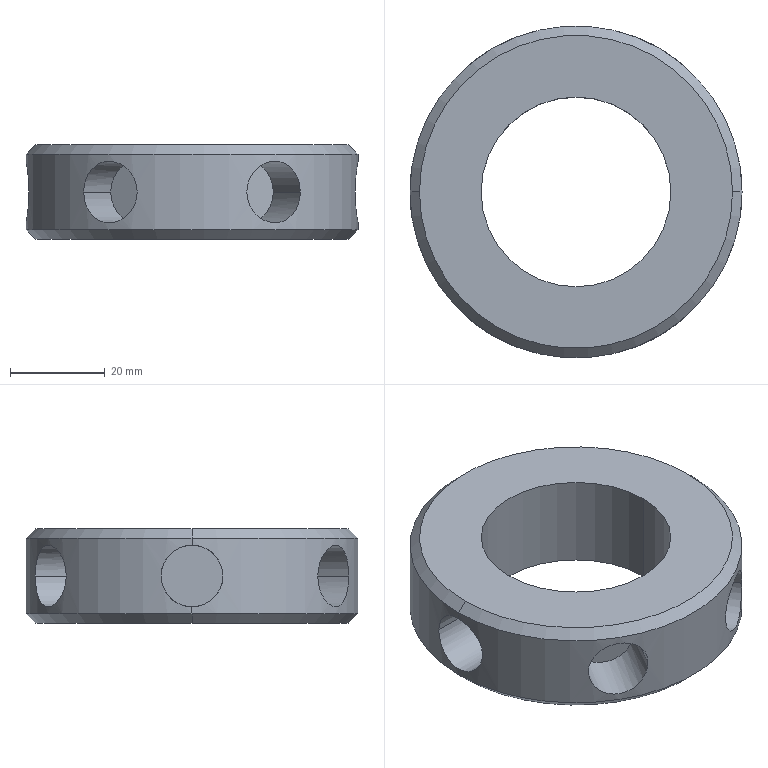Part | Creo | features CUT 6, DATUM PLANE 4, CURVE 2, CHAMFER 1, COORDINATE SYSTEM 1, PATTERN 1, PROTRUSION 1 | 1 solid | 28 faces | box 70 x 70 x 20 mm | volume 41537 mm3 | cylinder 16 | plane 8 | cone 4 | commonest cylinder face diameters 13 x12 40 x2 70 x2
STEP:
#1=CARTESIAN_POINT('',(0.,0.,0.));
#2=DIRECTION('',(0.,0.,1.));
#3=DIRECTION('',(1.,0.,0.));
#4=AXIS2_PLACEMENT_3D('',#1,#2,#3);
#5=CARTESIAN_POINT('',(-33.,0.,0.));
#6=VERTEX_POINT('',#5);
#7=CARTESIAN_POINT('',(33.,0.,0.));
#8=VERTEX_POINT('',#7);
#9=CARTESIAN_POINT('',(0.,0.,0.));
#10=DIRECTION('',(0.,0.,-1.));
#11=DIRECTION('',(-1.,0.,0.));
#12=AXIS2_PLACEMENT_3D('',#9,#10,#11);
#13=CIRCLE('',#12,33.);
#14=EDGE_CURVE('',#6,#8,#13,.T.);
#15=ORIENTED_EDGE('',*,*,#14,.F.);
#16=CARTESIAN_POINT('',(0.,0.,0.));
#17=DIRECTION('',(0.,0.,-1.));
#18=DIRECTION('',(1.,0.,0.));
#19=AXIS2_PLACEMENT_3D('',#16,#17,#18);
#20=CIRCLE('',#19,33.);
#21=EDGE_CURVE('',#8,#6,#20,.T.);
#22=ORIENTED_EDGE('',*,*,#21,.F.);
#23=EDGE_LOOP('',(#15,#22));
#24=FACE_OUTER_BOUND('',#23,.F.);
#25=CARTESIAN_POINT('',(20.,0.,0.));
#26=VERTEX_POINT('',#25);
#27=CARTESIAN_POINT('',(-20.,0.,0.));
#28=VERTEX_POINT('',#27);
#29=CARTESIAN_POINT('',(0.,0.,0.));
#30=DIRECTION('',(0.,0.,-1.));
#31=DIRECTION('',(1.,0.,0.));
#32=AXIS2_PLACEMENT_3D('',#29,#30,#31);
#33=CIRCLE('',#32,20.);
#34=EDGE_CURVE('',#26,#28,#33,.T.);
#35=ORIENTED_EDGE('',*,*,#34,.T.);
#36=CARTESIAN_POINT('',(0.,0.,0.));
#37=DIRECTION('',(0.,0.,-1.));
#38=DIRECTION('',(-1.,0.,0.));
#39=AXIS2_PLACEMENT_3D('',#36,#37,#38);
#40=CIRCLE('',#39,20.);
#41=EDGE_CURVE('',#28,#26,#40,.T.);
#42=ORIENTED_EDGE('',*,*,#41,.T.);
#43=EDGE_LOOP('',(#35,#42));
#44=FACE_BOUND('',#43,.F.);
#45=CARTESIAN_POINT('',(0.,0.,0.));
#46=DIRECTION('',(0.,0.,1.));
#47=DIRECTION('',(1.,0.,0.));
#48=AXIS2_PLACEMENT_3D('',#45,#46,#47);
#49=PLANE('',#48);
#50=ADVANCED_FACE('',(#24,#44),#49,.F.);
#51=ORIENTED_EDGE('',*,*,#34,.F.);
#52=CARTESIAN_POINT('',(20.,0.,20.));
#53=VERTEX_POINT('',#52);
#54=CARTESIAN_POINT('',(20.,0.,0.));
#55=DIRECTION('',(0.,0.,1.));
#56=VECTOR('',#55,20.);
#57=LINE('',#54,#56);
#58=EDGE_CURVE('',#26,#53,#57,.T.);
#59=ORIENTED_EDGE('',*,*,#58,.T.);
#60=CARTESIAN_POINT('',(-20.,0.,20.));
#61=VERTEX_POINT('',#60);
#62=CARTESIAN_POINT('',(0.,0.,20.));
#63=DIRECTION('',(0.,0.,-1.));
#64=DIRECTION('',(1.,0.,0.));
#65=AXIS2_PLACEMENT_3D('',#62,#63,#64);
#66=CIRCLE('',#65,20.);
#67=EDGE_CURVE('',#53,#61,#66,.T.);
#68=ORIENTED_EDGE('',*,*,#67,.T.);
#69=CARTESIAN_POINT('',(-20.,0.,0.));
#70=DIRECTION('',(0.,0.,1.));
#71=VECTOR('',#70,20.);
#72=LINE('',#69,#71);
#73=EDGE_CURVE('',#28,#61,#72,.T.);
#74=ORIENTED_EDGE('',*,*,#73,.F.);
#75=EDGE_LOOP('',(#51,#59,#68,#74));
#76=FACE_OUTER_BOUND('',#75,.F.);
#77=CARTESIAN_POINT('',(0.,0.,0.));
#78=DIRECTION('',(0.,0.,1.));
#79=DIRECTION('',(1.,0.,0.));
#80=AXIS2_PLACEMENT_3D('',#77,#78,#79);
#81=CYLINDRICAL_SURFACE('',#80,20.);
#82=ADVANCED_FACE('',(#76),#81,.F.);
#83=ORIENTED_EDGE('',*,*,#41,.F.);
#84=ORIENTED_EDGE('',*,*,#73,.T.);
#85=CARTESIAN_POINT('',(0.,0.,20.));
#86=DIRECTION('',(0.,0.,-1.));
#87=DIRECTION('',(-1.,0.,0.));
#88=AXIS2_PLACEMENT_3D('',#85,#86,#87);
#89=CIRCLE('',#88,20.);
#90=EDGE_CURVE('',#61,#53,#89,.T.);
#91=ORIENTED_EDGE('',*,*,#90,.T.);
#92=ORIENTED_EDGE('',*,*,#58,.F.);
#93=EDGE_LOOP('',(#83,#84,#91,#92));
#94=FACE_OUTER_BOUND('',#93,.F.);
#95=CARTESIAN_POINT('',(0.,0.,0.));
#96=DIRECTION('',(0.,0.,1.));
#97=DIRECTION('',(1.,0.,0.));
#98=AXIS2_PLACEMENT_3D('',#95,#96,#97);
#99=CYLINDRICAL_SURFACE('',#98,20.);
#100=ADVANCED_FACE('',(#94),#99,.F.);
#101=CARTESIAN_POINT('',(33.,0.,20.));
#102=VERTEX_POINT('',#101);
#103=CARTESIAN_POINT('',(-33.,0.,20.));
#104=VERTEX_POINT('',#103);
#105=CARTESIAN_POINT('',(0.,0.,20.));
#106=DIRECTION('',(0.,0.,1.));
#107=DIRECTION('',(1.,0.,0.));
#108=AXIS2_PLACEMENT_3D('',#105,#106,#107);
#109=CIRCLE('',#108,33.);
#110=EDGE_CURVE('',#102,#104,#109,.T.);
#111=ORIENTED_EDGE('',*,*,#110,.F.);
#112=CARTESIAN_POINT('',(0.,0.,20.));
#113=DIRECTION('',(0.,0.,1.));
#114=DIRECTION('',(-1.,0.,0.));
#115=AXIS2_PLACEMENT_3D('',#112,#113,#114);
#116=CIRCLE('',#115,33.);
#117=EDGE_CURVE('',#104,#102,#116,.T.);
#118=ORIENTED_EDGE('',*,*,#117,.F.);
#119=EDGE_LOOP('',(#111,#118));
#120=FACE_OUTER_BOUND('',#119,.F.);
#121=ORIENTED_EDGE('',*,*,#67,.F.);
#122=ORIENTED_EDGE('',*,*,#90,.F.);
#123=EDGE_LOOP('',(#121,#122));
#124=FACE_BOUND('',#123,.F.);
#125=CARTESIAN_POINT('',(0.,0.,20.));
#126=DIRECTION('',(0.,0.,1.));
#127=DIRECTION('',(1.,0.,0.));
#128=AXIS2_PLACEMENT_3D('',#125,#126,#127);
#129=PLANE('',#128);
#130=ADVANCED_FACE('',(#120,#124),#129,.T.);
#131=ORIENTED_EDGE('',*,*,#110,.T.);
#132=CARTESIAN_POINT('',(-35.,0.,18.));
#133=VERTEX_POINT('',#132);
#134=CARTESIAN_POINT('',(-33.,-0.000000004,20.));
#135=DIRECTION('',(-0.7071,0.,-0.7071));
#136=VECTOR('',#135,2.828);
#137=LINE('',#134,#136);
#138=EDGE_CURVE('',#104,#133,#137,.T.);
#139=ORIENTED_EDGE('',*,*,#138,.T.);
#140=CARTESIAN_POINT('',(35.,0.,18.));
#141=VERTEX_POINT('',#140);
#142=CARTESIAN_POINT('',(0.,0.,18.));
#143=DIRECTION('',(0.,0.,1.));
#144=DIRECTION('',(1.,0.,0.));
#145=AXIS2_PLACEMENT_3D('',#142,#143,#144);
#146=CIRCLE('',#145,35.);
#147=EDGE_CURVE('',#141,#133,#146,.T.);
#148=ORIENTED_EDGE('',*,*,#147,.F.);
#149=CARTESIAN_POINT('',(33.,0.000000004,20.));
#150=DIRECTION('',(0.7071,0.,-0.7071));
#151=VECTOR('',#150,2.828);
#152=LINE('',#149,#151);
#153=EDGE_CURVE('',#102,#141,#152,.T.);
#154=ORIENTED_EDGE('',*,*,#153,.F.);
#155=EDGE_LOOP('',(#131,#139,#148,#154));
#156=FACE_OUTER_BOUND('',#155,.F.);
#157=CARTESIAN_POINT('',(0.,0.,19.));
#158=DIRECTION('',(0.,0.,-1.));
#159=DIRECTION('',(0.,-1.,0.));
#160=AXIS2_PLACEMENT_3D('',#157,#158,#159);
#161=CONICAL_SURFACE('',#160,34.,45.);
#162=ADVANCED_FACE('',(#156),#161,.T.);
#163=ORIENTED_EDGE('',*,*,#117,.T.);
#164=ORIENTED_EDGE('',*,*,#153,.T.);
#165=CARTESIAN_POINT('',(0.,0.,18.));
#166=DIRECTION('',(0.,0.,1.));
#167=DIRECTION('',(-1.,0.,0.));
#168=AXIS2_PLACEMENT_3D('',#165,#166,#167);
#169=CIRCLE('',#168,35.);
#170=EDGE_CURVE('',#133,#141,#169,.T.);
#171=ORIENTED_EDGE('',*,*,#170,.F.);
#172=ORIENTED_EDGE('',*,*,#138,.F.);
#173=EDGE_LOOP('',(#163,#164,#171,#172));
#174=FACE_OUTER_BOUND('',#173,.F.);
#175=CARTESIAN_POINT('',(0.,0.,19.));
#176=DIRECTION('',(0.,0.,-1.));
#177=DIRECTION('',(0.,-1.,0.));
#178=AXIS2_PLACEMENT_3D('',#175,#176,#177);
#179=CONICAL_SURFACE('',#178,34.,45.);
#180=ADVANCED_FACE('',(#174),#179,.T.);
#181=CARTESIAN_POINT('',(35.,0.,2.));
#182=VERTEX_POINT('',#181);
#183=CARTESIAN_POINT('',(-35.,0.,2.));
#184=VERTEX_POINT('',#183);
#185=CARTESIAN_POINT('',(0.,0.,2.));
#186=DIRECTION('',(0.,0.,-1.));
#187=DIRECTION('',(1.,0.,0.));
#188=AXIS2_PLACEMENT_3D('',#185,#186,#187);
#189=CIRCLE('',#188,35.);
#190=EDGE_CURVE('',#182,#184,#189,.T.);
#191=ORIENTED_EDGE('',*,*,#190,.T.);
#192=CARTESIAN_POINT('',(-35.,0.,3.5));
#193=VERTEX_POINT('',#192);
#194=CARTESIAN_POINT('',(-35.,-0.000000003,2.));
#195=DIRECTION('',(0.,0.000000002,1.));
#196=VECTOR('',#195,1.5);
#197=LINE('',#194,#196);
#198=EDGE_CURVE('',#184,#193,#197,.T.);
#199=ORIENTED_EDGE('',*,*,#198,.T.);
#200=CARTESIAN_POINT('',(-34.391,-6.5,10.));
#201=VERTEX_POINT('',#200);
#202=CARTESIAN_POINT('',(-34.391,-6.5,9.619));
#203=CARTESIAN_POINT('',(-34.404,-6.434,8.869));
#204=CARTESIAN_POINT('',(-34.458,-6.137,7.76));
#205=CARTESIAN_POINT('',(-34.541,-5.658,6.734));
#206=CARTESIAN_POINT('',(-34.643,-5.001,5.796));
#207=CARTESIAN_POINT('',(-34.75,-4.205,5.001));
#208=CARTESIAN_POINT('',(-34.852,-3.269,4.343));
#209=CARTESIAN_POINT('',(-34.934,-2.239,3.862));
#210=CARTESIAN_POINT('',(-34.988,-1.113,3.562));
#211=CARTESIAN_POINT('',(-35.,-0.3734,3.5));
#212=CARTESIAN_POINT('',(-35.,0.,3.5));
#213=B_SPLINE_CURVE_WITH_KNOTS('',3,(#200,#202,#203,#204,#205,#206,#207,#208,#209,#210,#211,#212),.UNSPECIFIED.,.F.,.F.,(4,1,1,1,1,1,1,1,1,4),(0.,0.1111,0.2222,0.3333,0.4444,0.5556,0.6667,0.7778,0.8889,1.),.UNSPECIFIED.);
#214=EDGE_CURVE('',#201,#193,#213,.T.);
#215=ORIENTED_EDGE('',*,*,#214,.F.);
#216=CARTESIAN_POINT('',(-35.,0.,16.5));
#217=VERTEX_POINT('',#216);
#218=CARTESIAN_POINT('',(-35.,0.,16.5));
#219=CARTESIAN_POINT('',(-35.,-0.422,16.5));
#220=CARTESIAN_POINT('',(-34.985,-1.254,16.421));
#221=CARTESIAN_POINT('',(-34.917,-2.511,16.042));
#222=CARTESIAN_POINT('',(-34.816,-3.639,15.436));
#223=CARTESIAN_POINT('',(-34.697,-4.626,14.625));
#224=CARTESIAN_POINT('',(-34.578,-5.437,13.638));
#225=CARTESIAN_POINT('',(-34.476,-6.043,12.507));
#226=CARTESIAN_POINT('',(-34.407,-6.416,11.273));
#227=CARTESIAN_POINT('',(-34.391,-6.5,10.43));
#228=CARTESIAN_POINT('',(-34.391,-6.5,10.));
#229=B_SPLINE_CURVE_WITH_KNOTS('',3,(#218,#219,#220,#221,#222,#223,#224,#225,#226,#227,#228),.UNSPECIFIED.,.F.,.F.,(4,1,1,1,1,1,1,1,4),(0.,0.125,0.25,0.375,0.5,0.625,0.75,0.875,1.),.UNSPECIFIED.);
#230=EDGE_CURVE('',#217,#201,#229,.T.);
#231=ORIENTED_EDGE('',*,*,#230,.F.);
#232=CARTESIAN_POINT('',(-35.,0.,16.5));
#233=DIRECTION('',(0.,-0.000000002,1.));
#234=VECTOR('',#233,1.5);
#235=LINE('',#232,#234);
#236=EDGE_CURVE('',#217,#133,#235,.T.);
#237=ORIENTED_EDGE('',*,*,#236,.T.);
#238=ORIENTED_EDGE('',*,*,#170,.T.);
#239=CARTESIAN_POINT('',(35.,0.,16.5));
#240=VERTEX_POINT('',#239);
#241=CARTESIAN_POINT('',(35.,0.,16.5));
#242=DIRECTION('',(0.,0.000000002,1.));
#243=VECTOR('',#242,1.5);
#244=LINE('',#241,#243);
#245=EDGE_CURVE('',#240,#141,#244,.T.);
#246=ORIENTED_EDGE('',*,*,#245,.F.);
#247=CARTESIAN_POINT('',(34.391,-6.5,10.));
#248=VERTEX_POINT('',#247);
#249=CARTESIAN_POINT('',(34.391,-6.5,10.));
#250=CARTESIAN_POINT('',(34.391,-6.5,10.381));
#251=CARTESIAN_POINT('',(34.404,-6.434,11.131));
#252=CARTESIAN_POINT('',(34.458,-6.137,12.24));
#253=CARTESIAN_POINT('',(34.541,-5.658,13.266));
#254=CARTESIAN_POINT('',(34.643,-5.001,14.204));
#255=CARTESIAN_POINT('',(34.75,-4.205,14.999));
#256=CARTESIAN_POINT('',(34.852,-3.269,15.657));
#257=CARTESIAN_POINT('',(34.934,-2.239,16.138));
#258=CARTESIAN_POINT('',(34.988,-1.113,16.438));
#259=CARTESIAN_POINT('',(35.,-0.3732,16.5));
#260=CARTESIAN_POINT('',(35.,0.,16.5));
#261=B_SPLINE_CURVE_WITH_KNOTS('',3,(#249,#250,#251,#252,#253,#254,#255,#256,#257,#258,#259,#260),.UNSPECIFIED.,.F.,.F.,(4,1,1,1,1,1,1,1,1,4),(0.,0.1111,0.2222,0.3333,0.4444,0.5556,0.6667,0.7778,0.8889,1.),.UNSPECIFIED.);
#262=EDGE_CURVE('',#248,#240,#261,.T.);
#263=ORIENTED_EDGE('',*,*,#262,.F.);
#264=CARTESIAN_POINT('',(35.,0.,3.5));
#265=VERTEX_POINT('',#264);
#266=CARTESIAN_POINT('',(35.,0.,3.5));
#267=CARTESIAN_POINT('',(35.,-0.4219,3.5));
#268=CARTESIAN_POINT('',(34.985,-1.254,3.579));
#269=CARTESIAN_POINT('',(34.917,-2.511,3.958));
#270=CARTESIAN_POINT('',(34.816,-3.639,4.564));
#271=CARTESIAN_POINT('',(34.697,-4.626,5.375));
#272=CARTESIAN_POINT('',(34.578,-5.437,6.363));
#273=CARTESIAN_POINT('',(34.476,-6.043,7.493));
#274=CARTESIAN_POINT('',(34.407,-6.416,8.727));
#275=CARTESIAN_POINT('',(34.391,-6.5,9.57));
#276=B_SPLINE_CURVE_WITH_KNOTS('',3,(#266,#267,#268,#269,#270,#271,#272,#273,#274,#275,#247),.UNSPECIFIED.,.F.,.F.,(4,1,1,1,1,1,1,1,4),(0.,0.125,0.25,0.375,0.5,0.625,0.75,0.875,1.),.UNSPECIFIED.);
#277=EDGE_CURVE('',#265,#248,#276,.T.);
#278=ORIENTED_EDGE('',*,*,#277,.F.);
#279=CARTESIAN_POINT('',(35.,0.000000003,2.));
#280=DIRECTION('',(0.,-0.000000002,1.));
#281=VECTOR('',#280,1.5);
#282=LINE('',#279,#281);
#283=EDGE_CURVE('',#182,#265,#282,.T.);
#284=ORIENTED_EDGE('',*,*,#283,.F.);
#285=EDGE_LOOP('',(#191,#199,#215,#231,#237,#238,#246,#263,#278,#284));
#286=FACE_OUTER_BOUND('',#285,.F.);
#287=CARTESIAN_POINT('',(11.566,-33.034,10.));
#288=VERTEX_POINT('',#287);
#289=CARTESIAN_POINT('',(22.825,-26.534,10.));
#290=VERTEX_POINT('',#289);
#291=CARTESIAN_POINT('',(11.566,-33.034,9.544));
#292=CARTESIAN_POINT('',(11.657,-33.002,8.651));
#293=CARTESIAN_POINT('',(12.058,-32.859,7.348));
#294=CARTESIAN_POINT('',(12.708,-32.615,6.158));
#295=CARTESIAN_POINT('',(13.572,-32.267,5.132));
#296=CARTESIAN_POINT('',(14.6,-31.817,4.324));
#297=CARTESIAN_POINT('',(15.733,-31.274,3.769));
#298=CARTESIAN_POINT('',(16.913,-30.652,3.488));
#299=CARTESIAN_POINT('',(18.089,-29.973,3.488));
#300=CARTESIAN_POINT('',(19.218,-29.262,3.769));
#301=CARTESIAN_POINT('',(20.254,-28.552,4.324));
#302=CARTESIAN_POINT('',(21.158,-27.887,5.132));
#303=CARTESIAN_POINT('',(21.892,-27.313,6.158));
#304=CARTESIAN_POINT('',(22.428,-26.872,7.348));
#305=CARTESIAN_POINT('',(22.752,-26.596,8.651));
#306=CARTESIAN_POINT('',(22.825,-26.534,9.544));
#307=B_SPLINE_CURVE_WITH_KNOTS('',3,(#287,#291,#292,#293,#294,#295,#296,#297,#298,#299,#300,#301,#302,#303,#304,#305,#306,#289),.UNSPECIFIED.,.F.,.F.,(4,1,1,1,1,1,1,1,1,1,1,1,1,1,1,4),(0.,0.06667,0.1333,0.2,0.2667,0.3333,0.4,0.4667,0.5333,0.6,0.6667,0.7333,0.8,0.8667,0.9333,1.),.UNSPECIFIED.);
#308=EDGE_CURVE('',#288,#290,#307,.T.);
#309=ORIENTED_EDGE('',*,*,#308,.T.);
#310=CARTESIAN_POINT('',(22.825,-26.534,10.));
#311=CARTESIAN_POINT('',(22.825,-26.534,10.456));
#312=CARTESIAN_POINT('',(22.752,-26.596,11.349));
#313=CARTESIAN_POINT('',(22.428,-26.872,12.652));
#314=CARTESIAN_POINT('',(21.892,-27.313,13.842));
#315=CARTESIAN_POINT('',(21.158,-27.887,14.868));
#316=CARTESIAN_POINT('',(20.254,-28.552,15.676));
#317=CARTESIAN_POINT('',(19.218,-29.262,16.231));
#318=CARTESIAN_POINT('',(18.089,-29.973,16.512));
#319=CARTESIAN_POINT('',(16.913,-30.652,16.512));
#320=CARTESIAN_POINT('',(15.733,-31.274,16.231));
#321=CARTESIAN_POINT('',(14.6,-31.817,15.676));
#322=CARTESIAN_POINT('',(13.572,-32.267,14.868));
#323=CARTESIAN_POINT('',(12.708,-32.615,13.842));
#324=CARTESIAN_POINT('',(12.058,-32.859,12.652));
#325=CARTESIAN_POINT('',(11.657,-33.002,11.349));
#326=CARTESIAN_POINT('',(11.566,-33.034,10.456));
#327=CARTESIAN_POINT('',(11.566,-33.034,10.));
#328=B_SPLINE_CURVE_WITH_KNOTS('',3,(#310,#311,#312,#313,#314,#315,#316,#317,#318,#319,#320,#321,#322,#323,#324,#325,#326,#327),.UNSPECIFIED.,.F.,.F.,(4,1,1,1,1,1,1,1,1,1,1,1,1,1,1,4),(0.,0.06667,0.1333,0.2,0.2667,0.3333,0.4,0.4667,0.5333,0.6,0.6667,0.7333,0.8,0.8667,0.9333,1.),.UNSPECIFIED.);
#329=EDGE_CURVE('',#290,#288,#328,.T.);
#330=ORIENTED_EDGE('',*,*,#329,.T.);
#331=EDGE_LOOP('',(#309,#330));
#332=FACE_BOUND('',#331,.F.);
#333=CARTESIAN_POINT('',(-22.825,-26.534,10.));
#334=VERTEX_POINT('',#333);
#335=CARTESIAN_POINT('',(-11.566,-33.034,10.));
#336=VERTEX_POINT('',#335);
#337=CARTESIAN_POINT('',(-22.825,-26.534,9.544));
#338=CARTESIAN_POINT('',(-22.752,-26.596,8.651));
#339=CARTESIAN_POINT('',(-22.428,-26.872,7.348));
#340=CARTESIAN_POINT('',(-21.892,-27.313,6.158));
#341=CARTESIAN_POINT('',(-21.158,-27.887,5.132));
#342=CARTESIAN_POINT('',(-20.254,-28.552,4.324));
#343=CARTESIAN_POINT('',(-19.218,-29.262,3.769));
#344=CARTESIAN_POINT('',(-18.089,-29.973,3.488));
#345=CARTESIAN_POINT('',(-16.913,-30.652,3.488));
#346=CARTESIAN_POINT('',(-15.733,-31.274,3.769));
#347=CARTESIAN_POINT('',(-14.6,-31.817,4.324));
#348=CARTESIAN_POINT('',(-13.572,-32.267,5.132));
#349=CARTESIAN_POINT('',(-12.708,-32.615,6.158));
#350=CARTESIAN_POINT('',(-12.058,-32.859,7.348));
#351=CARTESIAN_POINT('',(-11.657,-33.002,8.651));
#352=CARTESIAN_POINT('',(-11.566,-33.034,9.544));
#353=B_SPLINE_CURVE_WITH_KNOTS('',3,(#333,#337,#338,#339,#340,#341,#342,#343,#344,#345,#346,#347,#348,#349,#350,#351,#352,#335),.UNSPECIFIED.,.F.,.F.,(4,1,1,1,1,1,1,1,1,1,1,1,1,1,1,4),(0.,0.06667,0.1333,0.2,0.2667,0.3333,0.4,0.4667,0.5333,0.6,0.6667,0.7333,0.8,0.8667,0.9333,1.),.UNSPECIFIED.);
#354=EDGE_CURVE('',#334,#336,#353,.T.);
#355=ORIENTED_EDGE('',*,*,#354,.T.);
#356=CARTESIAN_POINT('',(-11.566,-33.034,10.));
#357=CARTESIAN_POINT('',(-11.566,-33.034,10.456));
#358=CARTESIAN_POINT('',(-11.657,-33.002,11.349));
#359=CARTESIAN_POINT('',(-12.058,-32.859,12.652));
#360=CARTESIAN_POINT('',(-12.708,-32.615,13.842));
#361=CARTESIAN_POINT('',(-13.572,-32.267,14.868));
#362=CARTESIAN_POINT('',(-14.6,-31.817,15.676));
#363=CARTESIAN_POINT('',(-15.733,-31.274,16.231));
#364=CARTESIAN_POINT('',(-16.913,-30.652,16.512));
#365=CARTESIAN_POINT('',(-18.089,-29.973,16.512));
#366=CARTESIAN_POINT('',(-19.218,-29.262,16.231));
#367=CARTESIAN_POINT('',(-20.254,-28.552,15.676));
#368=CARTESIAN_POINT('',(-21.158,-27.887,14.868));
#369=CARTESIAN_POINT('',(-21.892,-27.313,13.842));
#370=CARTESIAN_POINT('',(-22.428,-26.872,12.652));
#371=CARTESIAN_POINT('',(-22.752,-26.596,11.349));
#372=CARTESIAN_POINT('',(-22.825,-26.534,10.456));
#373=CARTESIAN_POINT('',(-22.825,-26.534,10.));
#374=B_SPLINE_CURVE_WITH_KNOTS('',3,(#356,#357,#358,#359,#360,#361,#362,#363,#364,#365,#366,#367,#368,#369,#370,#371,#372,#373),.UNSPECIFIED.,.F.,.F.,(4,1,1,1,1,1,1,1,1,1,1,1,1,1,1,4),(0.,0.06667,0.1333,0.2,0.2667,0.3333,0.4,0.4667,0.5333,0.6,0.6667,0.7333,0.8,0.8667,0.9333,1.),.UNSPECIFIED.);
#375=EDGE_CURVE('',#336,#334,#374,.T.);
#376=ORIENTED_EDGE('',*,*,#375,.T.);
#377=EDGE_LOOP('',(#355,#376));
#378=FACE_BOUND('',#377,.F.);
#379=CARTESIAN_POINT('',(0.,0.,0.));
#380=DIRECTION('',(0.,0.,1.));
#381=DIRECTION('',(1.,0.,0.));
#382=AXIS2_PLACEMENT_3D('',#379,#380,#381);
#383=CYLINDRICAL_SURFACE('',#382,35.);
#384=ADVANCED_FACE('',(#286,#332,#378),#383,.T.);
#385=ORIENTED_EDGE('',*,*,#354,.F.);
#386=CARTESIAN_POINT('',(-17.129,-16.669,10.));
#387=VERTEX_POINT('',#386);
#388=CARTESIAN_POINT('',(-22.825,-26.534,10.));
#389=DIRECTION('',(0.5,0.866,0.));
#390=VECTOR('',#389,11.391);
#391=LINE('',#388,#390);
#392=EDGE_CURVE('',#334,#387,#391,.T.);
#393=ORIENTED_EDGE('',*,*,#392,.T.);
#394=CARTESIAN_POINT('',(-5.871,-23.169,10.));
#395=VERTEX_POINT('',#394);
#396=CARTESIAN_POINT('',(-11.5,-19.919,10.));
#397=DIRECTION('',(-0.5,-0.866,0.));
#398=DIRECTION('',(-0.866,0.5,0.));
#399=AXIS2_PLACEMENT_3D('',#396,#397,#398);
#400=CIRCLE('',#399,6.5);
#401=EDGE_CURVE('',#387,#395,#400,.T.);
#402=ORIENTED_EDGE('',*,*,#401,.T.);
#403=CARTESIAN_POINT('',(-11.566,-33.034,10.));
#404=DIRECTION('',(0.5,0.866,0.));
#405=VECTOR('',#404,11.391);
#406=LINE('',#403,#405);
#407=EDGE_CURVE('',#336,#395,#406,.T.);
#408=ORIENTED_EDGE('',*,*,#407,.F.);
#409=EDGE_LOOP('',(#385,#393,#402,#408));
#410=FACE_OUTER_BOUND('',#409,.F.);
#411=CARTESIAN_POINT('',(-17.5,-30.311,10.));
#412=DIRECTION('',(-0.5,-0.866,0.));
#413=DIRECTION('',(-0.866,0.5,0.));
#414=AXIS2_PLACEMENT_3D('',#411,#412,#413);
#415=CYLINDRICAL_SURFACE('',#414,6.5);
#416=ADVANCED_FACE('',(#410),#415,.F.);
#417=ORIENTED_EDGE('',*,*,#375,.F.);
#418=ORIENTED_EDGE('',*,*,#407,.T.);
#419=CARTESIAN_POINT('',(-11.5,-19.919,10.));
#420=DIRECTION('',(-0.5,-0.866,0.));
#421=DIRECTION('',(0.866,-0.5,0.));
#422=AXIS2_PLACEMENT_3D('',#419,#420,#421);
#423=CIRCLE('',#422,6.5);
#424=EDGE_CURVE('',#395,#387,#423,.T.);
#425=ORIENTED_EDGE('',*,*,#424,.T.);
#426=ORIENTED_EDGE('',*,*,#392,.F.);
#427=EDGE_LOOP('',(#417,#418,#425,#426));
#428=FACE_OUTER_BOUND('',#427,.F.);
#429=CARTESIAN_POINT('',(-17.5,-30.311,10.));
#430=DIRECTION('',(-0.5,-0.866,0.));
#431=DIRECTION('',(-0.866,0.5,0.));
#432=AXIS2_PLACEMENT_3D('',#429,#430,#431);
#433=CYLINDRICAL_SURFACE('',#432,6.5);
#434=ADVANCED_FACE('',(#428),#433,.F.);
#435=ORIENTED_EDGE('',*,*,#401,.F.);
#436=ORIENTED_EDGE('',*,*,#424,.F.);
#437=EDGE_LOOP('',(#435,#436));
#438=FACE_OUTER_BOUND('',#437,.F.);
#439=CARTESIAN_POINT('',(-11.5,-19.919,0.));
#440=DIRECTION('',(-0.5,-0.866,0.));
#441=DIRECTION('',(-0.866,0.5,0.));
#442=AXIS2_PLACEMENT_3D('',#439,#440,#441);
#443=PLANE('',#442);
#444=ADVANCED_FACE('',(#438),#443,.T.);
#445=ORIENTED_EDGE('',*,*,#308,.F.);
#446=CARTESIAN_POINT('',(5.871,-23.169,10.));
#447=VERTEX_POINT('',#446);
#448=CARTESIAN_POINT('',(11.566,-33.034,10.));
#449=DIRECTION('',(-0.5,0.866,0.));
#450=VECTOR('',#449,11.391);
#451=LINE('',#448,#450);
#452=EDGE_CURVE('',#288,#447,#451,.T.);
#453=ORIENTED_EDGE('',*,*,#452,.T.);
#454=CARTESIAN_POINT('',(17.129,-16.669,10.));
#455=VERTEX_POINT('',#454);
#456=CARTESIAN_POINT('',(11.5,-19.919,10.));
#457=DIRECTION('',(0.5,-0.866,0.));
#458=DIRECTION('',(-0.866,-0.5,0.));
#459=AXIS2_PLACEMENT_3D('',#456,#457,#458);
#460=CIRCLE('',#459,6.5);
#461=EDGE_CURVE('',#447,#455,#460,.T.);
#462=ORIENTED_EDGE('',*,*,#461,.T.);
#463=CARTESIAN_POINT('',(22.825,-26.534,10.));
#464=DIRECTION('',(-0.5,0.866,0.));
#465=VECTOR('',#464,11.391);
#466=LINE('',#463,#465);
#467=EDGE_CURVE('',#290,#455,#466,.T.);
#468=ORIENTED_EDGE('',*,*,#467,.F.);
#469=EDGE_LOOP('',(#445,#453,#462,#468));
#470=FACE_OUTER_BOUND('',#469,.F.);
#471=CARTESIAN_POINT('',(17.5,-30.311,10.));
#472=DIRECTION('',(0.5,-0.866,0.));
#473=DIRECTION('',(-0.866,-0.5,0.));
#474=AXIS2_PLACEMENT_3D('',#471,#472,#473);
#475=CYLINDRICAL_SURFACE('',#474,6.5);
#476=ADVANCED_FACE('',(#470),#475,.F.);
#477=ORIENTED_EDGE('',*,*,#329,.F.);
#478=ORIENTED_EDGE('',*,*,#467,.T.);
#479=CARTESIAN_POINT('',(11.5,-19.919,10.));
#480=DIRECTION('',(0.5,-0.866,0.));
#481=DIRECTION('',(0.866,0.5,0.));
#482=AXIS2_PLACEMENT_3D('',#479,#480,#481);
#483=CIRCLE('',#482,6.5);
#484=EDGE_CURVE('',#455,#447,#483,.T.);
#485=ORIENTED_EDGE('',*,*,#484,.T.);
#486=ORIENTED_EDGE('',*,*,#452,.F.);
#487=EDGE_LOOP('',(#477,#478,#485,#486));
#488=FACE_OUTER_BOUND('',#487,.F.);
#489=CARTESIAN_POINT('',(17.5,-30.311,10.));
#490=DIRECTION('',(0.5,-0.866,0.));
#491=DIRECTION('',(-0.866,-0.5,0.));
#492=AXIS2_PLACEMENT_3D('',#489,#490,#491);
#493=CYLINDRICAL_SURFACE('',#492,6.5);
#494=ADVANCED_FACE('',(#488),#493,.F.);
#495=ORIENTED_EDGE('',*,*,#461,.F.);
#496=ORIENTED_EDGE('',*,*,#484,.F.);
#497=EDGE_LOOP('',(#495,#496));
#498=FACE_OUTER_BOUND('',#497,.F.);
#499=CARTESIAN_POINT('',(11.5,-19.919,0.));
#500=DIRECTION('',(0.5,-0.866,0.));
#501=DIRECTION('',(-0.866,-0.5,0.));
#502=AXIS2_PLACEMENT_3D('',#499,#500,#501);
#503=PLANE('',#502);
#504=ADVANCED_FACE('',(#498),#503,.T.);
#505=ORIENTED_EDGE('',*,*,#21,.T.);
#506=CARTESIAN_POINT('',(-33.,-0.000000004,0.));
#507=DIRECTION('',(-0.7071,0.,0.7071));
#508=VECTOR('',#507,2.828);
#509=LINE('',#506,#508);
#510=EDGE_CURVE('',#6,#184,#509,.T.);
#511=ORIENTED_EDGE('',*,*,#510,.T.);
#512=ORIENTED_EDGE('',*,*,#190,.F.);
#513=CARTESIAN_POINT('',(33.,0.000000004,0.));
#514=DIRECTION('',(0.7071,0.,0.7071));
#515=VECTOR('',#514,2.828);
#516=LINE('',#513,#515);
#517=EDGE_CURVE('',#8,#182,#516,.T.);
#518=ORIENTED_EDGE('',*,*,#517,.F.);
#519=EDGE_LOOP('',(#505,#511,#512,#518));
#520=FACE_OUTER_BOUND('',#519,.F.);
#521=CARTESIAN_POINT('',(0.,0.,1.));
#522=DIRECTION('',(0.,0.,1.));
#523=DIRECTION('',(0.,-1.,0.));
#524=AXIS2_PLACEMENT_3D('',#521,#522,#523);
#525=CONICAL_SURFACE('',#524,34.,45.);
#526=ADVANCED_FACE('',(#520),#525,.T.);
#527=ORIENTED_EDGE('',*,*,#14,.T.);
#528=ORIENTED_EDGE('',*,*,#517,.T.);
#529=CARTESIAN_POINT('',(0.,0.,2.));
#530=DIRECTION('',(0.,0.,-1.));
#531=DIRECTION('',(-1.,0.,0.));
#532=AXIS2_PLACEMENT_3D('',#529,#530,#531);
#533=CIRCLE('',#532,35.);
#534=EDGE_CURVE('',#184,#182,#533,.T.);
#535=ORIENTED_EDGE('',*,*,#534,.F.);
#536=ORIENTED_EDGE('',*,*,#510,.F.);
#537=EDGE_LOOP('',(#527,#528,#535,#536));
#538=FACE_OUTER_BOUND('',#537,.F.);
#539=CARTESIAN_POINT('',(0.,0.,1.));
#540=DIRECTION('',(0.,0.,1.));
#541=DIRECTION('',(0.,-1.,0.));
#542=AXIS2_PLACEMENT_3D('',#539,#540,#541);
#543=CONICAL_SURFACE('',#542,34.,45.);
#544=ADVANCED_FACE('',(#538),#543,.T.);
#545=ORIENTED_EDGE('',*,*,#534,.T.);
#546=ORIENTED_EDGE('',*,*,#283,.T.);
#547=CARTESIAN_POINT('',(34.391,6.5,10.));
#548=VERTEX_POINT('',#547);
#549=CARTESIAN_POINT('',(34.391,6.5,9.619));
#550=CARTESIAN_POINT('',(34.404,6.434,8.869));
#551=CARTESIAN_POINT('',(34.458,6.137,7.76));
#552=CARTESIAN_POINT('',(34.541,5.658,6.734));
#553=CARTESIAN_POINT('',(34.643,5.001,5.796));
#554=CARTESIAN_POINT('',(34.75,4.205,5.001));
#555=CARTESIAN_POINT('',(34.852,3.269,4.343));
#556=CARTESIAN_POINT('',(34.934,2.239,3.862));
#557=CARTESIAN_POINT('',(34.988,1.113,3.562));
#558=CARTESIAN_POINT('',(35.,0.3734,3.5));
#559=B_SPLINE_CURVE_WITH_KNOTS('',3,(#547,#549,#550,#551,#552,#553,#554,#555,#556,#557,#558,#264),.UNSPECIFIED.,.F.,.F.,(4,1,1,1,1,1,1,1,1,4),(0.,0.1111,0.2222,0.3333,0.4444,0.5556,0.6667,0.7778,0.8889,1.),.UNSPECIFIED.);
#560=EDGE_CURVE('',#548,#265,#559,.T.);
#561=ORIENTED_EDGE('',*,*,#560,.F.);
#562=CARTESIAN_POINT('',(35.,0.422,16.5));
#563=CARTESIAN_POINT('',(34.985,1.254,16.421));
#564=CARTESIAN_POINT('',(34.917,2.511,16.042));
#565=CARTESIAN_POINT('',(34.816,3.639,15.436));
#566=CARTESIAN_POINT('',(34.697,4.626,14.625));
#567=CARTESIAN_POINT('',(34.578,5.437,13.638));
#568=CARTESIAN_POINT('',(34.476,6.043,12.507));
#569=CARTESIAN_POINT('',(34.407,6.416,11.273));
#570=CARTESIAN_POINT('',(34.391,6.5,10.43));
#571=CARTESIAN_POINT('',(34.391,6.5,10.));
#572=B_SPLINE_CURVE_WITH_KNOTS('',3,(#239,#562,#563,#564,#565,#566,#567,#568,#569,#570,#571),.UNSPECIFIED.,.F.,.F.,(4,1,1,1,1,1,1,1,4),(0.,0.125,0.25,0.375,0.5,0.625,0.75,0.875,1.),.UNSPECIFIED.);
#573=EDGE_CURVE('',#240,#548,#572,.T.);
#574=ORIENTED_EDGE('',*,*,#573,.F.);
#575=ORIENTED_EDGE('',*,*,#245,.T.);
#576=ORIENTED_EDGE('',*,*,#147,.T.);
#577=ORIENTED_EDGE('',*,*,#236,.F.);
#578=CARTESIAN_POINT('',(-34.391,6.5,10.));
#579=VERTEX_POINT('',#578);
#580=CARTESIAN_POINT('',(-34.391,6.5,10.));
#581=CARTESIAN_POINT('',(-34.391,6.5,10.381));
#582=CARTESIAN_POINT('',(-34.404,6.434,11.131));
#583=CARTESIAN_POINT('',(-34.458,6.137,12.24));
#584=CARTESIAN_POINT('',(-34.541,5.658,13.266));
#585=CARTESIAN_POINT('',(-34.643,5.001,14.204));
#586=CARTESIAN_POINT('',(-34.75,4.205,14.999));
#587=CARTESIAN_POINT('',(-34.852,3.269,15.657));
#588=CARTESIAN_POINT('',(-34.934,2.239,16.138));
#589=CARTESIAN_POINT('',(-34.988,1.113,16.438));
#590=CARTESIAN_POINT('',(-35.,0.3732,16.5));
#591=B_SPLINE_CURVE_WITH_KNOTS('',3,(#580,#581,#582,#583,#584,#585,#586,#587,#588,#589,#590,#216),.UNSPECIFIED.,.F.,.F.,(4,1,1,1,1,1,1,1,1,4),(0.,0.1111,0.2222,0.3333,0.4444,0.5556,0.6667,0.7778,0.8889,1.),.UNSPECIFIED.);
#592=EDGE_CURVE('',#579,#217,#591,.T.);
#593=ORIENTED_EDGE('',*,*,#592,.F.);
#594=CARTESIAN_POINT('',(-35.,0.4219,3.5));
#595=CARTESIAN_POINT('',(-34.985,1.254,3.579));
#596=CARTESIAN_POINT('',(-34.917,2.511,3.958));
#597=CARTESIAN_POINT('',(-34.816,3.639,4.564));
#598=CARTESIAN_POINT('',(-34.697,4.626,5.375));
#599=CARTESIAN_POINT('',(-34.578,5.437,6.363));
#600=CARTESIAN_POINT('',(-34.476,6.043,7.493));
#601=CARTESIAN_POINT('',(-34.407,6.416,8.727));
#602=CARTESIAN_POINT('',(-34.391,6.5,9.57));
#603=B_SPLINE_CURVE_WITH_KNOTS('',3,(#192,#594,#595,#596,#597,#598,#599,#600,#601,#602,#578),.UNSPECIFIED.,.F.,.F.,(4,1,1,1,1,1,1,1,4),(0.,0.125,0.25,0.375,0.5,0.625,0.75,0.875,1.),.UNSPECIFIED.);
#604=EDGE_CURVE('',#193,#579,#603,.T.);
#605=ORIENTED_EDGE('',*,*,#604,.F.);
#606=ORIENTED_EDGE('',*,*,#198,.F.);
#607=EDGE_LOOP('',(#545,#546,#561,#574,#575,#576,#577,#593,#605,#606));
#608=FACE_OUTER_BOUND('',#607,.F.);
#609=CARTESIAN_POINT('',(-11.566,33.034,10.));
#610=VERTEX_POINT('',#609);
#611=CARTESIAN_POINT('',(-22.825,26.534,10.));
#612=VERTEX_POINT('',#611);
#613=CARTESIAN_POINT('',(-11.566,33.034,9.544));
#614=CARTESIAN_POINT('',(-11.657,33.002,8.651));
#615=CARTESIAN_POINT('',(-12.058,32.859,7.348));
#616=CARTESIAN_POINT('',(-12.708,32.615,6.158));
#617=CARTESIAN_POINT('',(-13.572,32.267,5.132));
#618=CARTESIAN_POINT('',(-14.6,31.817,4.324));
#619=CARTESIAN_POINT('',(-15.733,31.274,3.769));
#620=CARTESIAN_POINT('',(-16.913,30.652,3.488));
#621=CARTESIAN_POINT('',(-18.089,29.973,3.488));
#622=CARTESIAN_POINT('',(-19.218,29.262,3.769));
#623=CARTESIAN_POINT('',(-20.254,28.552,4.324));
#624=CARTESIAN_POINT('',(-21.158,27.887,5.132));
#625=CARTESIAN_POINT('',(-21.892,27.313,6.158));
#626=CARTESIAN_POINT('',(-22.428,26.872,7.348));
#627=CARTESIAN_POINT('',(-22.752,26.596,8.651));
#628=CARTESIAN_POINT('',(-22.825,26.534,9.544));
#629=B_SPLINE_CURVE_WITH_KNOTS('',3,(#609,#613,#614,#615,#616,#617,#618,#619,#620,#621,#622,#623,#624,#625,#626,#627,#628,#611),.UNSPECIFIED.,.F.,.F.,(4,1,1,1,1,1,1,1,1,1,1,1,1,1,1,4),(0.,0.06667,0.1333,0.2,0.2667,0.3333,0.4,0.4667,0.5333,0.6,0.6667,0.7333,0.8,0.8667,0.9333,1.),.UNSPECIFIED.);
#630=EDGE_CURVE('',#610,#612,#629,.T.);
#631=ORIENTED_EDGE('',*,*,#630,.T.);
#632=CARTESIAN_POINT('',(-22.825,26.534,10.));
#633=CARTESIAN_POINT('',(-22.825,26.534,10.456));
#634=CARTESIAN_POINT('',(-22.752,26.596,11.349));
#635=CARTESIAN_POINT('',(-22.428,26.872,12.652));
#636=CARTESIAN_POINT('',(-21.892,27.313,13.842));
#637=CARTESIAN_POINT('',(-21.158,27.887,14.868));
#638=CARTESIAN_POINT('',(-20.254,28.552,15.676));
#639=CARTESIAN_POINT('',(-19.218,29.262,16.231));
#640=CARTESIAN_POINT('',(-18.089,29.973,16.512));
#641=CARTESIAN_POINT('',(-16.913,30.652,16.512));
#642=CARTESIAN_POINT('',(-15.733,31.274,16.231));
#643=CARTESIAN_POINT('',(-14.6,31.817,15.676));
#644=CARTESIAN_POINT('',(-13.572,32.267,14.868));
#645=CARTESIAN_POINT('',(-12.708,32.615,13.842));
#646=CARTESIAN_POINT('',(-12.058,32.859,12.652));
#647=CARTESIAN_POINT('',(-11.657,33.002,11.349));
#648=CARTESIAN_POINT('',(-11.566,33.034,10.456));
#649=CARTESIAN_POINT('',(-11.566,33.034,10.));
#650=B_SPLINE_CURVE_WITH_KNOTS('',3,(#632,#633,#634,#635,#636,#637,#638,#639,#640,#641,#642,#643,#644,#645,#646,#647,#648,#649),.UNSPECIFIED.,.F.,.F.,(4,1,1,1,1,1,1,1,1,1,1,1,1,1,1,4),(0.,0.06667,0.1333,0.2,0.2667,0.3333,0.4,0.4667,0.5333,0.6,0.6667,0.7333,0.8,0.8667,0.9333,1.),.UNSPECIFIED.);
#651=EDGE_CURVE('',#612,#610,#650,.T.);
#652=ORIENTED_EDGE('',*,*,#651,.T.);
#653=EDGE_LOOP('',(#631,#652));
#654=FACE_BOUND('',#653,.F.);
#655=CARTESIAN_POINT('',(22.825,26.534,10.));
#656=VERTEX_POINT('',#655);
#657=CARTESIAN_POINT('',(11.566,33.034,10.));
#658=VERTEX_POINT('',#657);
#659=CARTESIAN_POINT('',(22.825,26.534,9.544));
#660=CARTESIAN_POINT('',(22.752,26.596,8.651));
#661=CARTESIAN_POINT('',(22.428,26.872,7.348));
#662=CARTESIAN_POINT('',(21.892,27.313,6.158));
#663=CARTESIAN_POINT('',(21.158,27.887,5.132));
#664=CARTESIAN_POINT('',(20.254,28.552,4.324));
#665=CARTESIAN_POINT('',(19.218,29.262,3.769));
#666=CARTESIAN_POINT('',(18.089,29.973,3.488));
#667=CARTESIAN_POINT('',(16.913,30.652,3.488));
#668=CARTESIAN_POINT('',(15.733,31.274,3.769));
#669=CARTESIAN_POINT('',(14.6,31.817,4.324));
#670=CARTESIAN_POINT('',(13.572,32.267,5.132));
#671=CARTESIAN_POINT('',(12.708,32.615,6.158));
#672=CARTESIAN_POINT('',(12.058,32.859,7.348));
#673=CARTESIAN_POINT('',(11.657,33.002,8.651));
#674=CARTESIAN_POINT('',(11.566,33.034,9.544));
#675=B_SPLINE_CURVE_WITH_KNOTS('',3,(#655,#659,#660,#661,#662,#663,#664,#665,#666,#667,#668,#669,#670,#671,#672,#673,#674,#657),.UNSPECIFIED.,.F.,.F.,(4,1,1,1,1,1,1,1,1,1,1,1,1,1,1,4),(0.,0.06667,0.1333,0.2,0.2667,0.3333,0.4,0.4667,0.5333,0.6,0.6667,0.7333,0.8,0.8667,0.9333,1.),.UNSPECIFIED.);
#676=EDGE_CURVE('',#656,#658,#675,.T.);
#677=ORIENTED_EDGE('',*,*,#676,.T.);
#678=CARTESIAN_POINT('',(11.566,33.034,10.));
#679=CARTESIAN_POINT('',(11.566,33.034,10.456));
#680=CARTESIAN_POINT('',(11.657,33.002,11.349));
#681=CARTESIAN_POINT('',(12.058,32.859,12.652));
#682=CARTESIAN_POINT('',(12.708,32.615,13.842));
#683=CARTESIAN_POINT('',(13.572,32.267,14.868));
#684=CARTESIAN_POINT('',(14.6,31.817,15.676));
#685=CARTESIAN_POINT('',(15.733,31.274,16.231));
#686=CARTESIAN_POINT('',(16.913,30.652,16.512));
#687=CARTESIAN_POINT('',(18.089,29.973,16.512));
#688=CARTESIAN_POINT('',(19.218,29.262,16.231));
#689=CARTESIAN_POINT('',(20.254,28.552,15.676));
#690=CARTESIAN_POINT('',(21.158,27.887,14.868));
#691=CARTESIAN_POINT('',(21.892,27.313,13.842));
#692=CARTESIAN_POINT('',(22.428,26.872,12.652));
#693=CARTESIAN_POINT('',(22.752,26.596,11.349));
#694=CARTESIAN_POINT('',(22.825,26.534,10.456));
#695=CARTESIAN_POINT('',(22.825,26.534,10.));
#696=B_SPLINE_CURVE_WITH_KNOTS('',3,(#678,#679,#680,#681,#682,#683,#684,#685,#686,#687,#688,#689,#690,#691,#692,#693,#694,#695),.UNSPECIFIED.,.F.,.F.,(4,1,1,1,1,1,1,1,1,1,1,1,1,1,1,4),(0.,0.06667,0.1333,0.2,0.2667,0.3333,0.4,0.4667,0.5333,0.6,0.6667,0.7333,0.8,0.8667,0.9333,1.),.UNSPECIFIED.);
#697=EDGE_CURVE('',#658,#656,#696,.T.);
#698=ORIENTED_EDGE('',*,*,#697,.T.);
#699=EDGE_LOOP('',(#677,#698));
#700=FACE_BOUND('',#699,.F.);
#701=CARTESIAN_POINT('',(0.,0.,0.));
#702=DIRECTION('',(0.,0.,1.));
#703=DIRECTION('',(1.,0.,0.));
#704=AXIS2_PLACEMENT_3D('',#701,#702,#703);
#705=CYLINDRICAL_SURFACE('',#704,35.);
#706=ADVANCED_FACE('',(#608,#654,#700),#705,.T.);
#707=ORIENTED_EDGE('',*,*,#676,.F.);
#708=CARTESIAN_POINT('',(17.129,16.669,10.));
#709=VERTEX_POINT('',#708);
#710=CARTESIAN_POINT('',(22.825,26.534,10.));
#711=DIRECTION('',(-0.5,-0.866,0.));
#712=VECTOR('',#711,11.391);
#713=LINE('',#710,#712);
#714=EDGE_CURVE('',#656,#709,#713,.T.);
#715=ORIENTED_EDGE('',*,*,#714,.T.);
#716=CARTESIAN_POINT('',(5.871,23.169,10.));
#717=VERTEX_POINT('',#716);
#718=CARTESIAN_POINT('',(11.5,19.919,10.));
#719=DIRECTION('',(0.5,0.866,0.));
#720=DIRECTION('',(0.866,-0.5,0.));
#721=AXIS2_PLACEMENT_3D('',#718,#719,#720);
#722=CIRCLE('',#721,6.5);
#723=EDGE_CURVE('',#709,#717,#722,.T.);
#724=ORIENTED_EDGE('',*,*,#723,.T.);
#725=CARTESIAN_POINT('',(11.566,33.034,10.));
#726=DIRECTION('',(-0.5,-0.866,0.));
#727=VECTOR('',#726,11.391);
#728=LINE('',#725,#727);
#729=EDGE_CURVE('',#658,#717,#728,.T.);
#730=ORIENTED_EDGE('',*,*,#729,.F.);
#731=EDGE_LOOP('',(#707,#715,#724,#730));
#732=FACE_OUTER_BOUND('',#731,.F.);
#733=CARTESIAN_POINT('',(17.5,30.311,10.));
#734=DIRECTION('',(0.5,0.866,0.));
#735=DIRECTION('',(0.866,-0.5,0.));
#736=AXIS2_PLACEMENT_3D('',#733,#734,#735);
#737=CYLINDRICAL_SURFACE('',#736,6.5);
#738=ADVANCED_FACE('',(#732),#737,.F.);
#739=ORIENTED_EDGE('',*,*,#697,.F.);
#740=ORIENTED_EDGE('',*,*,#729,.T.);
#741=CARTESIAN_POINT('',(11.5,19.919,10.));
#742=DIRECTION('',(0.5,0.866,0.));
#743=DIRECTION('',(-0.866,0.5,0.));
#744=AXIS2_PLACEMENT_3D('',#741,#742,#743);
#745=CIRCLE('',#744,6.5);
#746=EDGE_CURVE('',#717,#709,#745,.T.);
#747=ORIENTED_EDGE('',*,*,#746,.T.);
#748=ORIENTED_EDGE('',*,*,#714,.F.);
#749=EDGE_LOOP('',(#739,#740,#747,#748));
#750=FACE_OUTER_BOUND('',#749,.F.);
#751=CARTESIAN_POINT('',(17.5,30.311,10.));
#752=DIRECTION('',(0.5,0.866,0.));
#753=DIRECTION('',(0.866,-0.5,0.));
#754=AXIS2_PLACEMENT_3D('',#751,#752,#753);
#755=CYLINDRICAL_SURFACE('',#754,6.5);
#756=ADVANCED_FACE('',(#750),#755,.F.);
#757=ORIENTED_EDGE('',*,*,#723,.F.);
#758=ORIENTED_EDGE('',*,*,#746,.F.);
#759=EDGE_LOOP('',(#757,#758));
#760=FACE_OUTER_BOUND('',#759,.F.);
#761=CARTESIAN_POINT('',(11.5,19.919,0.));
#762=DIRECTION('',(0.5,0.866,0.));
#763=DIRECTION('',(0.866,-0.5,0.));
#764=AXIS2_PLACEMENT_3D('',#761,#762,#763);
#765=PLANE('',#764);
#766=ADVANCED_FACE('',(#760),#765,.T.);
#767=ORIENTED_EDGE('',*,*,#630,.F.);
#768=CARTESIAN_POINT('',(-5.871,23.169,10.));
#769=VERTEX_POINT('',#768);
#770=CARTESIAN_POINT('',(-11.566,33.034,10.));
#771=DIRECTION('',(0.5,-0.866,0.));
#772=VECTOR('',#771,11.391);
#773=LINE('',#770,#772);
#774=EDGE_CURVE('',#610,#769,#773,.T.);
#775=ORIENTED_EDGE('',*,*,#774,.T.);
#776=CARTESIAN_POINT('',(-17.129,16.669,10.));
#777=VERTEX_POINT('',#776);
#778=CARTESIAN_POINT('',(-11.5,19.919,10.));
#779=DIRECTION('',(-0.5,0.866,0.));
#780=DIRECTION('',(0.866,0.5,0.));
#781=AXIS2_PLACEMENT_3D('',#778,#779,#780);
#782=CIRCLE('',#781,6.5);
#783=EDGE_CURVE('',#769,#777,#782,.T.);
#784=ORIENTED_EDGE('',*,*,#783,.T.);
#785=CARTESIAN_POINT('',(-22.825,26.534,10.));
#786=DIRECTION('',(0.5,-0.866,0.));
#787=VECTOR('',#786,11.391);
#788=LINE('',#785,#787);
#789=EDGE_CURVE('',#612,#777,#788,.T.);
#790=ORIENTED_EDGE('',*,*,#789,.F.);
#791=EDGE_LOOP('',(#767,#775,#784,#790));
#792=FACE_OUTER_BOUND('',#791,.F.);
#793=CARTESIAN_POINT('',(-17.5,30.311,10.));
#794=DIRECTION('',(-0.5,0.866,0.));
#795=DIRECTION('',(0.866,0.5,0.));
#796=AXIS2_PLACEMENT_3D('',#793,#794,#795);
#797=CYLINDRICAL_SURFACE('',#796,6.5);
#798=ADVANCED_FACE('',(#792),#797,.F.);
#799=ORIENTED_EDGE('',*,*,#651,.F.);
#800=ORIENTED_EDGE('',*,*,#789,.T.);
#801=CARTESIAN_POINT('',(-11.5,19.919,10.));
#802=DIRECTION('',(-0.5,0.866,0.));
#803=DIRECTION('',(-0.866,-0.5,0.));
#804=AXIS2_PLACEMENT_3D('',#801,#802,#803);
#805=CIRCLE('',#804,6.5);
#806=EDGE_CURVE('',#777,#769,#805,.T.);
#807=ORIENTED_EDGE('',*,*,#806,.T.);
#808=ORIENTED_EDGE('',*,*,#774,.F.);
#809=EDGE_LOOP('',(#799,#800,#807,#808));
#810=FACE_OUTER_BOUND('',#809,.F.);
#811=CARTESIAN_POINT('',(-17.5,30.311,10.));
#812=DIRECTION('',(-0.5,0.866,0.));
#813=DIRECTION('',(0.866,0.5,0.));
#814=AXIS2_PLACEMENT_3D('',#811,#812,#813);
#815=CYLINDRICAL_SURFACE('',#814,6.5);
#816=ADVANCED_FACE('',(#810),#815,.F.);
#817=ORIENTED_EDGE('',*,*,#783,.F.);
#818=ORIENTED_EDGE('',*,*,#806,.F.);
#819=EDGE_LOOP('',(#817,#818));
#820=FACE_OUTER_BOUND('',#819,.F.);
#821=CARTESIAN_POINT('',(-11.5,19.919,0.));
#822=DIRECTION('',(-0.5,0.866,0.));
#823=DIRECTION('',(0.866,0.5,0.));
#824=AXIS2_PLACEMENT_3D('',#821,#822,#823);
#825=PLANE('',#824);
#826=ADVANCED_FACE('',(#820),#825,.T.);
#827=ORIENTED_EDGE('',*,*,#560,.T.);
#828=ORIENTED_EDGE('',*,*,#277,.T.);
#829=CARTESIAN_POINT('',(23.,-6.5,10.));
#830=VERTEX_POINT('',#829);
#831=CARTESIAN_POINT('',(34.391,-6.5,10.));
#832=DIRECTION('',(-1.,0.,0.));
#833=VECTOR('',#832,11.391);
#834=LINE('',#831,#833);
#835=EDGE_CURVE('',#248,#830,#834,.T.);
#836=ORIENTED_EDGE('',*,*,#835,.T.);
#837=CARTESIAN_POINT('',(23.,6.5,10.));
#838=VERTEX_POINT('',#837);
#839=CARTESIAN_POINT('',(23.,0.,10.));
#840=DIRECTION('',(1.,0.,0.));
#841=DIRECTION('',(0.,-1.,0.));
#842=AXIS2_PLACEMENT_3D('',#839,#840,#841);
#843=CIRCLE('',#842,6.5);
#844=EDGE_CURVE('',#830,#838,#843,.T.);
#845=ORIENTED_EDGE('',*,*,#844,.T.);
#846=CARTESIAN_POINT('',(34.391,6.5,10.));
#847=DIRECTION('',(-1.,0.,0.));
#848=VECTOR('',#847,11.391);
#849=LINE('',#846,#848);
#850=EDGE_CURVE('',#548,#838,#849,.T.);
#851=ORIENTED_EDGE('',*,*,#850,.F.);
#852=EDGE_LOOP('',(#827,#828,#836,#845,#851));
#853=FACE_OUTER_BOUND('',#852,.F.);
#854=CARTESIAN_POINT('',(35.,0.,10.));
#855=DIRECTION('',(1.,0.,0.));
#856=DIRECTION('',(0.,-1.,0.));
#857=AXIS2_PLACEMENT_3D('',#854,#855,#856);
#858=CYLINDRICAL_SURFACE('',#857,6.5);
#859=ADVANCED_FACE('',(#853),#858,.F.);
#860=ORIENTED_EDGE('',*,*,#573,.T.);
#861=ORIENTED_EDGE('',*,*,#850,.T.);
#862=CARTESIAN_POINT('',(23.,0.,10.));
#863=DIRECTION('',(1.,0.,0.));
#864=DIRECTION('',(0.,1.,0.));
#865=AXIS2_PLACEMENT_3D('',#862,#863,#864);
#866=CIRCLE('',#865,6.5);
#867=EDGE_CURVE('',#838,#830,#866,.T.);
#868=ORIENTED_EDGE('',*,*,#867,.T.);
#869=ORIENTED_EDGE('',*,*,#835,.F.);
#870=ORIENTED_EDGE('',*,*,#262,.T.);
#871=EDGE_LOOP('',(#860,#861,#868,#869,#870));
#872=FACE_OUTER_BOUND('',#871,.F.);
#873=CARTESIAN_POINT('',(35.,0.,10.));
#874=DIRECTION('',(1.,0.,0.));
#875=DIRECTION('',(0.,-1.,0.));
#876=AXIS2_PLACEMENT_3D('',#873,#874,#875);
#877=CYLINDRICAL_SURFACE('',#876,6.5);
#878=ADVANCED_FACE('',(#872),#877,.F.);
#879=ORIENTED_EDGE('',*,*,#844,.F.);
#880=ORIENTED_EDGE('',*,*,#867,.F.);
#881=EDGE_LOOP('',(#879,#880));
#882=FACE_OUTER_BOUND('',#881,.F.);
#883=CARTESIAN_POINT('',(23.,0.,0.));
#884=DIRECTION('',(1.,0.,0.));
#885=DIRECTION('',(0.,-1.,0.));
#886=AXIS2_PLACEMENT_3D('',#883,#884,#885);
#887=PLANE('',#886);
#888=ADVANCED_FACE('',(#882),#887,.T.);
#889=ORIENTED_EDGE('',*,*,#592,.T.);
#890=ORIENTED_EDGE('',*,*,#230,.T.);
#891=CARTESIAN_POINT('',(-23.,-6.5,10.));
#892=VERTEX_POINT('',#891);
#893=CARTESIAN_POINT('',(-34.391,-6.5,10.));
#894=DIRECTION('',(1.,0.,0.));
#895=VECTOR('',#894,11.391);
#896=LINE('',#893,#895);
#897=EDGE_CURVE('',#201,#892,#896,.T.);
#898=ORIENTED_EDGE('',*,*,#897,.T.);
#899=CARTESIAN_POINT('',(-23.,6.5,10.));
#900=VERTEX_POINT('',#899);
#901=CARTESIAN_POINT('',(-23.,0.,10.));
#902=DIRECTION('',(-1.,0.,0.));
#903=DIRECTION('',(0.,-1.,0.));
#904=AXIS2_PLACEMENT_3D('',#901,#902,#903);
#905=CIRCLE('',#904,6.5);
#906=EDGE_CURVE('',#892,#900,#905,.T.);
#907=ORIENTED_EDGE('',*,*,#906,.T.);
#908=CARTESIAN_POINT('',(-34.391,6.5,10.));
#909=DIRECTION('',(1.,0.,0.));
#910=VECTOR('',#909,11.391);
#911=LINE('',#908,#910);
#912=EDGE_CURVE('',#579,#900,#911,.T.);
#913=ORIENTED_EDGE('',*,*,#912,.F.);
#914=EDGE_LOOP('',(#889,#890,#898,#907,#913));
#915=FACE_OUTER_BOUND('',#914,.F.);
#916=CARTESIAN_POINT('',(-35.,0.,10.));
#917=DIRECTION('',(-1.,0.,0.));
#918=DIRECTION('',(0.,1.,0.));
#919=AXIS2_PLACEMENT_3D('',#916,#917,#918);
#920=CYLINDRICAL_SURFACE('',#919,6.5);
#921=ADVANCED_FACE('',(#915),#920,.F.);
#922=ORIENTED_EDGE('',*,*,#604,.T.);
#923=ORIENTED_EDGE('',*,*,#912,.T.);
#924=CARTESIAN_POINT('',(-23.,0.,10.));
#925=DIRECTION('',(-1.,0.,0.));
#926=DIRECTION('',(0.,1.,0.));
#927=AXIS2_PLACEMENT_3D('',#924,#925,#926);
#928=CIRCLE('',#927,6.5);
#929=EDGE_CURVE('',#900,#892,#928,.T.);
#930=ORIENTED_EDGE('',*,*,#929,.T.);
#931=ORIENTED_EDGE('',*,*,#897,.F.);
#932=ORIENTED_EDGE('',*,*,#214,.T.);
#933=EDGE_LOOP('',(#922,#923,#930,#931,#932));
#934=FACE_OUTER_BOUND('',#933,.F.);
#935=CARTESIAN_POINT('',(-35.,0.,10.));
#936=DIRECTION('',(-1.,0.,0.));
#937=DIRECTION('',(0.,1.,0.));
#938=AXIS2_PLACEMENT_3D('',#935,#936,#937);
#939=CYLINDRICAL_SURFACE('',#938,6.5);
#940=ADVANCED_FACE('',(#934),#939,.F.);
#941=ORIENTED_EDGE('',*,*,#929,.F.);
#942=ORIENTED_EDGE('',*,*,#906,.F.);
#943=EDGE_LOOP('',(#941,#942));
#944=FACE_OUTER_BOUND('',#943,.F.);
#945=CARTESIAN_POINT('',(-23.,0.,0.));
#946=DIRECTION('',(-1.,0.,0.));
#947=DIRECTION('',(0.,1.,0.));
#948=AXIS2_PLACEMENT_3D('',#945,#946,#947);
#949=PLANE('',#948);
#950=ADVANCED_FACE('',(#944),#949,.T.);
#951=CLOSED_SHELL('',(#50,#82,#100,#130,#162,#180,#384,#416,#434,#444,#476,#494,#504,#526,#544,#706,#738,#756,#766,#798,#816,#826,#859,#878,#888,#921,#940,#950));
#952=MANIFOLD_SOLID_BREP('',#951);
#953=(LENGTH_UNIT()NAMED_UNIT(*)SI_UNIT(.MILLI.,.METRE.));
#954=UNCERTAINTY_MEASURE_WITH_UNIT(LENGTH_MEASURE(0.0101),#953,'','');
#955=(NAMED_UNIT(*)PLANE_ANGLE_UNIT()SI_UNIT($,.RADIAN.));
#956=PLANE_ANGLE_MEASURE_WITH_UNIT(PLANE_ANGLE_MEASURE(0.01745),#955);
#957=(CONVERSION_BASED_UNIT('DEGREE',#956)NAMED_UNIT(*)PLANE_ANGLE_UNIT());
#958=(NAMED_UNIT(*)SI_UNIT($,.STERADIAN.)SOLID_ANGLE_UNIT());
#959=(GEOMETRIC_REPRESENTATION_CONTEXT(3)GLOBAL_UNCERTAINTY_ASSIGNED_CONTEXT((#954))GLOBAL_UNIT_ASSIGNED_CONTEXT((#953,#957,#958))REPRESENTATION_CONTEXT('',''));
#960=ADVANCED_BREP_SHAPE_REPRESENTATION('',(#4,#952),#959);